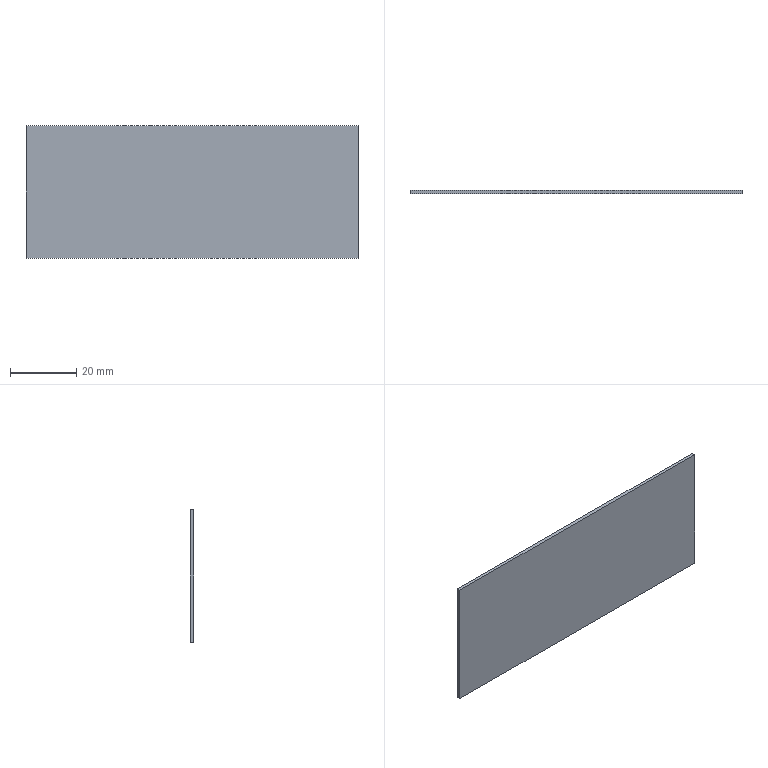Part | SolidWorks | features MirrorStock 1 | 1 solid | 6 faces | box 100 x 1 x 40 mm | volume 4000 mm3 | plane 6
STEP:
#1=CARTESIAN_POINT('',(50.,0.,-20.));
#2=VERTEX_POINT('',#1);
#3=CARTESIAN_POINT('',(50.,0.,20.));
#4=VERTEX_POINT('',#3);
#5=CARTESIAN_POINT('',(50.,0.,-20.));
#6=DIRECTION('',(0.,0.,1.));
#7=VECTOR('',#6,1000.);
#8=LINE('',#5,#7);
#9=EDGE_CURVE('',#2,#4,#8,.T.);
#10=ORIENTED_EDGE('',*,*,#9,.F.);
#11=CARTESIAN_POINT('',(50.,1.,-20.));
#12=VERTEX_POINT('',#11);
#13=CARTESIAN_POINT('',(50.,1.,-20.));
#14=DIRECTION('',(0.,-1.,0.));
#15=VECTOR('',#14,1000.);
#16=LINE('',#13,#15);
#17=EDGE_CURVE('',#12,#2,#16,.T.);
#18=ORIENTED_EDGE('',*,*,#17,.F.);
#19=CARTESIAN_POINT('',(50.,1.,20.));
#20=VERTEX_POINT('',#19);
#21=CARTESIAN_POINT('',(50.,1.,-20.));
#22=DIRECTION('',(0.,0.,1.));
#23=VECTOR('',#22,1000.);
#24=LINE('',#21,#23);
#25=EDGE_CURVE('',#12,#20,#24,.T.);
#26=ORIENTED_EDGE('',*,*,#25,.T.);
#27=CARTESIAN_POINT('',(50.,1.,20.));
#28=DIRECTION('',(0.,-1.,0.));
#29=VECTOR('',#28,1000.);
#30=LINE('',#27,#29);
#31=EDGE_CURVE('',#20,#4,#30,.T.);
#32=ORIENTED_EDGE('',*,*,#31,.T.);
#33=EDGE_LOOP('',(#10,#18,#26,#32));
#34=FACE_OUTER_BOUND('',#33,.T.);
#35=CARTESIAN_POINT('',(50.,1.,-20.));
#36=DIRECTION('',(-1.,0.,0.));
#37=DIRECTION('',(0.,0.,-1.));
#38=AXIS2_PLACEMENT_3D('',#35,#36,#37);
#39=PLANE('',#38);
#40=ADVANCED_FACE('',(#34),#39,.F.);
#41=CARTESIAN_POINT('',(-50.,0.,20.));
#42=VERTEX_POINT('',#41);
#43=CARTESIAN_POINT('',(-50.,0.,20.));
#44=DIRECTION('',(-1.,0.,0.));
#45=VECTOR('',#44,1000.);
#46=LINE('',#43,#45);
#47=EDGE_CURVE('',#4,#42,#46,.T.);
#48=ORIENTED_EDGE('',*,*,#47,.F.);
#49=ORIENTED_EDGE('',*,*,#31,.F.);
#50=CARTESIAN_POINT('',(-50.,1.,20.));
#51=VERTEX_POINT('',#50);
#52=CARTESIAN_POINT('',(-50.,1.,20.));
#53=DIRECTION('',(-1.,0.,0.));
#54=VECTOR('',#53,1000.);
#55=LINE('',#52,#54);
#56=EDGE_CURVE('',#20,#51,#55,.T.);
#57=ORIENTED_EDGE('',*,*,#56,.T.);
#58=CARTESIAN_POINT('',(-50.,1.,20.));
#59=DIRECTION('',(0.,-1.,0.));
#60=VECTOR('',#59,1000.);
#61=LINE('',#58,#60);
#62=EDGE_CURVE('',#51,#42,#61,.T.);
#63=ORIENTED_EDGE('',*,*,#62,.T.);
#64=EDGE_LOOP('',(#48,#49,#57,#63));
#65=FACE_OUTER_BOUND('',#64,.T.);
#66=CARTESIAN_POINT('',(-50.,1.,20.));
#67=DIRECTION('',(0.,0.,-1.));
#68=DIRECTION('',(1.,0.,0.));
#69=AXIS2_PLACEMENT_3D('',#66,#67,#68);
#70=PLANE('',#69);
#71=ADVANCED_FACE('',(#65),#70,.F.);
#72=CARTESIAN_POINT('',(-50.,0.,-20.));
#73=VERTEX_POINT('',#72);
#74=CARTESIAN_POINT('',(-50.,0.,-20.));
#75=DIRECTION('',(0.,0.,-1.));
#76=VECTOR('',#75,1000.);
#77=LINE('',#74,#76);
#78=EDGE_CURVE('',#42,#73,#77,.T.);
#79=ORIENTED_EDGE('',*,*,#78,.F.);
#80=ORIENTED_EDGE('',*,*,#62,.F.);
#81=CARTESIAN_POINT('',(-50.,1.,-20.));
#82=VERTEX_POINT('',#81);
#83=CARTESIAN_POINT('',(-50.,1.,-20.));
#84=DIRECTION('',(0.,0.,-1.));
#85=VECTOR('',#84,1000.);
#86=LINE('',#83,#85);
#87=EDGE_CURVE('',#51,#82,#86,.T.);
#88=ORIENTED_EDGE('',*,*,#87,.T.);
#89=CARTESIAN_POINT('',(-50.,1.,-20.));
#90=DIRECTION('',(0.,-1.,0.));
#91=VECTOR('',#90,1000.);
#92=LINE('',#89,#91);
#93=EDGE_CURVE('',#82,#73,#92,.T.);
#94=ORIENTED_EDGE('',*,*,#93,.T.);
#95=EDGE_LOOP('',(#79,#80,#88,#94));
#96=FACE_OUTER_BOUND('',#95,.T.);
#97=CARTESIAN_POINT('',(-50.,1.,-20.));
#98=DIRECTION('',(1.,0.,0.));
#99=DIRECTION('',(0.,0.,1.));
#100=AXIS2_PLACEMENT_3D('',#97,#98,#99);
#101=PLANE('',#100);
#102=ADVANCED_FACE('',(#96),#101,.F.);
#103=CARTESIAN_POINT('',(-50.,0.,-20.));
#104=DIRECTION('',(1.,0.,0.));
#105=VECTOR('',#104,1000.);
#106=LINE('',#103,#105);
#107=EDGE_CURVE('',#73,#2,#106,.T.);
#108=ORIENTED_EDGE('',*,*,#107,.F.);
#109=ORIENTED_EDGE('',*,*,#93,.F.);
#110=CARTESIAN_POINT('',(-50.,1.,-20.));
#111=DIRECTION('',(1.,0.,0.));
#112=VECTOR('',#111,1000.);
#113=LINE('',#110,#112);
#114=EDGE_CURVE('',#82,#12,#113,.T.);
#115=ORIENTED_EDGE('',*,*,#114,.T.);
#116=ORIENTED_EDGE('',*,*,#17,.T.);
#117=EDGE_LOOP('',(#108,#109,#115,#116));
#118=FACE_OUTER_BOUND('',#117,.T.);
#119=CARTESIAN_POINT('',(-50.,1.,-20.));
#120=DIRECTION('',(0.,0.,1.));
#121=DIRECTION('',(-1.,0.,0.));
#122=AXIS2_PLACEMENT_3D('',#119,#120,#121);
#123=PLANE('',#122);
#124=ADVANCED_FACE('',(#118),#123,.F.);
#125=ORIENTED_EDGE('',*,*,#25,.F.);
#126=ORIENTED_EDGE('',*,*,#114,.F.);
#127=ORIENTED_EDGE('',*,*,#87,.F.);
#128=ORIENTED_EDGE('',*,*,#56,.F.);
#129=EDGE_LOOP('',(#125,#126,#127,#128));
#130=FACE_OUTER_BOUND('',#129,.T.);
#131=CARTESIAN_POINT('',(0.,1.,0.));
#132=DIRECTION('',(0.,-1.,0.));
#133=DIRECTION('',(0.,0.,1.));
#134=AXIS2_PLACEMENT_3D('',#131,#132,#133);
#135=PLANE('',#134);
#136=ADVANCED_FACE('',(#130),#135,.F.);
#137=ORIENTED_EDGE('',*,*,#9,.T.);
#138=ORIENTED_EDGE('',*,*,#47,.T.);
#139=ORIENTED_EDGE('',*,*,#78,.T.);
#140=ORIENTED_EDGE('',*,*,#107,.T.);
#141=EDGE_LOOP('',(#137,#138,#139,#140));
#142=FACE_OUTER_BOUND('',#141,.T.);
#143=CARTESIAN_POINT('',(0.,0.,0.));
#144=DIRECTION('',(0.,-1.,0.));
#145=DIRECTION('',(0.,0.,1.));
#146=AXIS2_PLACEMENT_3D('',#143,#144,#145);
#147=PLANE('',#146);
#148=ADVANCED_FACE('',(#142),#147,.T.);
#149=CLOSED_SHELL('',(#40,#71,#102,#124,#136,#148));
#150=MANIFOLD_SOLID_BREP('',#149);
#151=CARTESIAN_POINT('',(0.,0.,0.));
#152=DIRECTION('',(0.,0.,1.));
#153=DIRECTION('',(1.,0.,0.));
#154=AXIS2_PLACEMENT_3D('',#151,#152,#153);
#155=(LENGTH_UNIT()NAMED_UNIT(*)SI_UNIT(.MILLI.,.METRE.));
#156=UNCERTAINTY_MEASURE_WITH_UNIT(LENGTH_MEASURE(0.00001),#155,'','');
#157=(NAMED_UNIT(*)PLANE_ANGLE_UNIT()SI_UNIT($,.RADIAN.));
#158=(NAMED_UNIT(*)SI_UNIT($,.STERADIAN.)SOLID_ANGLE_UNIT());
#159=(GEOMETRIC_REPRESENTATION_CONTEXT(3)GLOBAL_UNCERTAINTY_ASSIGNED_CONTEXT((#156))GLOBAL_UNIT_ASSIGNED_CONTEXT((#155,#157,#158))REPRESENTATION_CONTEXT('',''));
#160=ADVANCED_BREP_SHAPE_REPRESENTATION('',(#150,#154),#159);